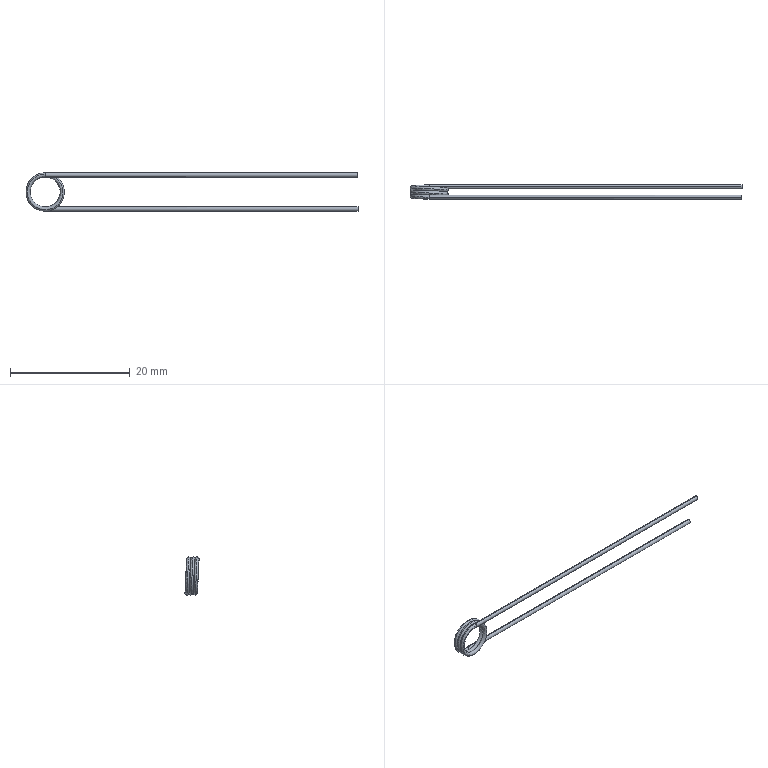Part | SolidWorks | features MoveFace 2, CompositeCurve 1, Helix 1, Sweep 1 | 1 solid | 9 faces | box 55.45 x 2.45 x 6.4 mm | volume 56.865 mm3 | cylinder 4 | spline 3 | plane 2 | commonest cylinder face diameters 0.7 x4
STEP:
#1=CARTESIAN_POINT('',(52.25,1.75,-3.2));
#2=VERTEX_POINT('',#1);
#3=CARTESIAN_POINT('',(52.25,1.75,-2.5));
#4=VERTEX_POINT('',#3);
#5=CARTESIAN_POINT('',(52.25,1.75,-2.85));
#6=DIRECTION('',(1.,0.,0.));
#7=DIRECTION('',(0.,0.00009155,-1.));
#8=AXIS2_PLACEMENT_3D('',#5,#6,#7);
#9=CIRCLE('',#8,0.35);
#10=EDGE_CURVE('',#2,#4,#9,.T.);
#11=ORIENTED_EDGE('',*,*,#10,.F.);
#12=CARTESIAN_POINT('',(-0.000000536,1.75,-3.2));
#13=VERTEX_POINT('',#12);
#14=CARTESIAN_POINT('',(12.85,1.75,-3.2));
#15=DIRECTION('',(-1.,0.,0.));
#16=VECTOR('',#15,1000.);
#17=LINE('',#14,#16);
#18=EDGE_CURVE('',#2,#13,#17,.T.);
#19=ORIENTED_EDGE('',*,*,#18,.T.);
#20=CARTESIAN_POINT('',(-0.006305,2.074,-2.979));
#21=VERTEX_POINT('',#20);
#22=CARTESIAN_POINT('',(0.,1.75,-2.85));
#23=DIRECTION('',(1.,0.,0.));
#24=DIRECTION('',(0.,0.00009155,-1.));
#25=AXIS2_PLACEMENT_3D('',#22,#23,#24);
#26=CIRCLE('',#25,0.35);
#27=EDGE_CURVE('',#13,#21,#26,.T.);
#28=ORIENTED_EDGE('',*,*,#27,.T.);
#29=CARTESIAN_POINT('',(0.,1.75,-2.5));
#30=VERTEX_POINT('',#29);
#31=CARTESIAN_POINT('',(0.,1.75,-2.85));
#32=DIRECTION('',(1.,0.,0.));
#33=DIRECTION('',(0.,0.00009155,-1.));
#34=AXIS2_PLACEMENT_3D('',#31,#32,#33);
#35=CIRCLE('',#34,0.35);
#36=EDGE_CURVE('',#21,#30,#35,.T.);
#37=ORIENTED_EDGE('',*,*,#36,.T.);
#38=CARTESIAN_POINT('',(12.85,1.75,-2.5));
#39=DIRECTION('',(-1.,0.,0.));
#40=VECTOR('',#39,1000.);
#41=LINE('',#38,#40);
#42=EDGE_CURVE('',#4,#30,#41,.T.);
#43=ORIENTED_EDGE('',*,*,#42,.F.);
#44=EDGE_LOOP('',(#11,#19,#28,#37,#43));
#45=FACE_OUTER_BOUND('',#44,.T.);
#46=CARTESIAN_POINT('',(12.85,1.75,-2.85));
#47=DIRECTION('',(-1.,0.,0.));
#48=DIRECTION('',(0.,0.,1.));
#49=AXIS2_PLACEMENT_3D('',#46,#47,#48);
#50=CYLINDRICAL_SURFACE('',#49,0.35);
#51=ADVANCED_FACE('',(#45),#50,.T.);
#52=CARTESIAN_POINT('',(0.006305,0.3239,2.979));
#53=VERTEX_POINT('',#52);
#54=CARTESIAN_POINT('',(0.,0.,3.2));
#55=VERTEX_POINT('',#54);
#56=CARTESIAN_POINT('',(0.006305,0.3239,2.979));
#57=CARTESIAN_POINT('',(0.01048,0.2681,3.104));
#58=CARTESIAN_POINT('',(0.005425,0.1388,3.2));
#59=CARTESIAN_POINT('',(0.,0.,3.2));
#60=B_SPLINE_CURVE_WITH_KNOTS('',3,(#56,#57,#58,#59),.UNSPECIFIED.,.F.,.F.,(4,4),(0.00002721,0.1895),.UNSPECIFIED.);
#61=EDGE_CURVE('',#53,#55,#60,.T.);
#62=ORIENTED_EDGE('',*,*,#61,.T.);
#63=CARTESIAN_POINT('',(52.25,0.,3.2));
#64=VERTEX_POINT('',#63);
#65=CARTESIAN_POINT('',(0.,0.,3.2));
#66=DIRECTION('',(1.,0.,0.));
#67=VECTOR('',#66,1000.);
#68=LINE('',#65,#67);
#69=EDGE_CURVE('',#55,#64,#68,.T.);
#70=ORIENTED_EDGE('',*,*,#69,.T.);
#71=CARTESIAN_POINT('',(52.25,0.,2.5));
#72=VERTEX_POINT('',#71);
#73=CARTESIAN_POINT('',(52.25,0.,2.85));
#74=DIRECTION('',(-1.,0.,0.));
#75=DIRECTION('',(0.,0.,1.));
#76=AXIS2_PLACEMENT_3D('',#73,#74,#75);
#77=CIRCLE('',#76,0.35);
#78=EDGE_CURVE('',#64,#72,#77,.T.);
#79=ORIENTED_EDGE('',*,*,#78,.T.);
#80=CARTESIAN_POINT('',(0.,0.,2.5));
#81=VERTEX_POINT('',#80);
#82=CARTESIAN_POINT('',(0.,0.,2.5));
#83=DIRECTION('',(1.,0.,0.));
#84=VECTOR('',#83,1000.);
#85=LINE('',#82,#84);
#86=EDGE_CURVE('',#81,#72,#85,.T.);
#87=ORIENTED_EDGE('',*,*,#86,.F.);
#88=CARTESIAN_POINT('',(0.,0.,2.85));
#89=DIRECTION('',(-1.,0.,0.));
#90=DIRECTION('',(0.,0.,1.));
#91=AXIS2_PLACEMENT_3D('',#88,#89,#90);
#92=CIRCLE('',#91,0.35);
#93=EDGE_CURVE('',#53,#81,#92,.T.);
#94=ORIENTED_EDGE('',*,*,#93,.F.);
#95=EDGE_LOOP('',(#62,#70,#79,#87,#94));
#96=FACE_OUTER_BOUND('',#95,.T.);
#97=CARTESIAN_POINT('',(0.,0.,2.85));
#98=DIRECTION('',(1.,0.,0.));
#99=DIRECTION('',(0.,0.,-1.));
#100=AXIS2_PLACEMENT_3D('',#97,#98,#99);
#101=CYLINDRICAL_SURFACE('',#100,0.35);
#102=ADVANCED_FACE('',(#96),#101,.T.);
#103=ORIENTED_EDGE('',*,*,#18,.F.);
#104=CARTESIAN_POINT('',(52.25,1.75,-2.85));
#105=DIRECTION('',(1.,0.,0.));
#106=DIRECTION('',(0.,0.00009155,-1.));
#107=AXIS2_PLACEMENT_3D('',#104,#105,#106);
#108=CIRCLE('',#107,0.35);
#109=EDGE_CURVE('',#4,#2,#108,.T.);
#110=ORIENTED_EDGE('',*,*,#109,.F.);
#111=ORIENTED_EDGE('',*,*,#42,.T.);
#112=CARTESIAN_POINT('',(0.006304,1.426,-2.979));
#113=VERTEX_POINT('',#112);
#114=CARTESIAN_POINT('',(0.,1.75,-2.85));
#115=DIRECTION('',(1.,0.,0.));
#116=DIRECTION('',(0.,0.00009155,-1.));
#117=AXIS2_PLACEMENT_3D('',#114,#115,#116);
#118=CIRCLE('',#117,0.35);
#119=EDGE_CURVE('',#30,#113,#118,.T.);
#120=ORIENTED_EDGE('',*,*,#119,.T.);
#121=CARTESIAN_POINT('',(0.,1.75,-2.85));
#122=DIRECTION('',(1.,0.,0.));
#123=DIRECTION('',(0.,0.00009155,-1.));
#124=AXIS2_PLACEMENT_3D('',#121,#122,#123);
#125=CIRCLE('',#124,0.35);
#126=EDGE_CURVE('',#113,#13,#125,.T.);
#127=ORIENTED_EDGE('',*,*,#126,.T.);
#128=EDGE_LOOP('',(#103,#110,#111,#120,#127));
#129=FACE_OUTER_BOUND('',#128,.T.);
#130=CARTESIAN_POINT('',(12.85,1.75,-2.85));
#131=DIRECTION('',(-1.,0.,0.));
#132=DIRECTION('',(0.,0.,1.));
#133=AXIS2_PLACEMENT_3D('',#130,#131,#132);
#134=CYLINDRICAL_SURFACE('',#133,0.35);
#135=ADVANCED_FACE('',(#129),#134,.T.);
#136=ORIENTED_EDGE('',*,*,#36,.F.);
#137=CARTESIAN_POINT('',(0.006305,0.3239,2.979));
#138=CARTESIAN_POINT('',(-0.7712,0.3519,2.981));
#139=CARTESIAN_POINT('',(-1.545,0.381,2.663));
#140=CARTESIAN_POINT('',(-2.649,0.4392,1.566));
#141=CARTESIAN_POINT('',(-2.975,0.4683,0.7939));
#142=CARTESIAN_POINT('',(-2.98,0.5195,-0.5733));
#143=CARTESIAN_POINT('',(-2.806,0.5413,-1.156));
#144=CARTESIAN_POINT('',(-2.162,0.585,-2.13));
#145=CARTESIAN_POINT('',(-1.69,0.6069,-2.521));
#146=CARTESIAN_POINT('',(-0.4324,0.658,-3.048));
#147=CARTESIAN_POINT('',(0.405,0.6871,-3.052));
#148=CARTESIAN_POINT('',(1.67,0.7383,-2.534));
#149=CARTESIAN_POINT('',(2.142,0.7601,-2.15));
#150=CARTESIAN_POINT('',(2.795,0.8037,-1.182));
#151=CARTESIAN_POINT('',(2.976,0.8257,-0.5972));
#152=CARTESIAN_POINT('',(2.981,0.8768,0.7668));
#153=CARTESIAN_POINT('',(2.665,0.9058,1.542));
#154=CARTESIAN_POINT('',(1.702,0.957,2.513));
#155=CARTESIAN_POINT('',(1.167,0.9788,2.801));
#156=CARTESIAN_POINT('',(0.02248,1.022,3.035));
#157=CARTESIAN_POINT('',(-0.587,1.044,2.978));
#158=CARTESIAN_POINT('',(-1.849,1.096,2.461));
#159=CARTESIAN_POINT('',(-2.445,1.125,1.872));
#160=CARTESIAN_POINT('',(-2.973,1.176,0.6109));
#161=CARTESIAN_POINT('',(-3.035,1.198,0.005944));
#162=CARTESIAN_POINT('',(-2.812,1.241,-1.14));
#163=CARTESIAN_POINT('',(-2.526,1.263,-1.682));
#164=CARTESIAN_POINT('',(-1.566,1.314,-2.65));
#165=CARTESIAN_POINT('',(-0.7938,1.343,-2.975));
#166=CARTESIAN_POINT('',(0.5733,1.395,-2.98));
#167=CARTESIAN_POINT('',(1.156,1.416,-2.806));
#168=CARTESIAN_POINT('',(2.13,1.46,-2.162));
#169=CARTESIAN_POINT('',(2.521,1.482,-1.69));
#170=CARTESIAN_POINT('',(3.048,1.533,-0.4324));
#171=CARTESIAN_POINT('',(3.052,1.562,0.405));
#172=CARTESIAN_POINT('',(2.534,1.613,1.67));
#173=CARTESIAN_POINT('',(2.15,1.635,2.142));
#174=CARTESIAN_POINT('',(1.182,1.679,2.795));
#175=CARTESIAN_POINT('',(0.5972,1.701,2.976));
#176=CARTESIAN_POINT('',(-0.7668,1.752,2.981));
#177=CARTESIAN_POINT('',(-1.542,1.781,2.665));
#178=CARTESIAN_POINT('',(-2.513,1.832,1.702));
#179=CARTESIAN_POINT('',(-2.801,1.854,1.167));
#180=CARTESIAN_POINT('',(-3.034,1.897,0.0225));
#181=CARTESIAN_POINT('',(-2.978,1.919,-0.587));
#182=CARTESIAN_POINT('',(-2.46,1.971,-1.85));
#183=CARTESIAN_POINT('',(-1.872,2.,-2.445));
#184=CARTESIAN_POINT('',(-0.7917,2.043,-2.897));
#185=CARTESIAN_POINT('',(-0.4042,2.058,-2.976));
#186=CARTESIAN_POINT('',(-0.006305,2.074,-2.979));
#187=B_SPLINE_CURVE_WITH_KNOTS('',3,(#137,#138,#139,#140,#141,#142,#143,#144,#145,#146,#147,#148,#149,#150,#151,#152,#153,#154,#155,#156,#157,#158,#159,#160,#161,#162,#163,#164,#165,#166,#167,#168,#169,#170,#171,#172,#173,#174,#175,#176,#177,#178,#179,#180,#181,#182,#183,#184,#185,#186),.UNSPECIFIED.,.F.,.F.,(4,2,2,2,2,2,2,2,2,2,2,2,2,2,2,2,2,2,2,2,2,2,2,2,4),(0.,0.04998,0.09999,0.1375,0.175,0.225,0.2625,0.3,0.35,0.3875,0.425,0.475,0.5125,0.55,0.6,0.6375,0.675,0.725,0.7625,0.8,0.85,0.8875,0.925,0.975,1.),.UNSPECIFIED.);
#188=EDGE_CURVE('',#53,#21,#187,.T.);
#189=ORIENTED_EDGE('',*,*,#188,.F.);
#190=ORIENTED_EDGE('',*,*,#93,.T.);
#191=CARTESIAN_POINT('',(-0.006304,-0.3239,2.979));
#192=VERTEX_POINT('',#191);
#193=CARTESIAN_POINT('',(0.,0.,2.85));
#194=DIRECTION('',(-1.,0.,0.));
#195=DIRECTION('',(0.,0.,1.));
#196=AXIS2_PLACEMENT_3D('',#193,#194,#195);
#197=CIRCLE('',#196,0.35);
#198=EDGE_CURVE('',#81,#192,#197,.T.);
#199=ORIENTED_EDGE('',*,*,#198,.T.);
#200=CARTESIAN_POINT('',(0.006304,1.426,-2.979));
#201=CARTESIAN_POINT('',(-0.379,1.413,-2.98));
#202=CARTESIAN_POINT('',(-0.7673,1.398,-2.904));
#203=CARTESIAN_POINT('',(-1.851,1.354,-2.461));
#204=CARTESIAN_POINT('',(-2.445,1.325,-1.871));
#205=CARTESIAN_POINT('',(-2.973,1.274,-0.6122));
#206=CARTESIAN_POINT('',(-3.035,1.252,-0.003211));
#207=CARTESIAN_POINT('',(-2.811,1.209,1.143));
#208=CARTESIAN_POINT('',(-2.527,1.187,1.681));
#209=CARTESIAN_POINT('',(-1.565,1.136,2.652));
#210=CARTESIAN_POINT('',(-0.792,1.107,2.975));
#211=CARTESIAN_POINT('',(0.572,1.056,2.981));
#212=CARTESIAN_POINT('',(1.158,1.034,2.805));
#213=CARTESIAN_POINT('',(2.132,0.99,2.16));
#214=CARTESIAN_POINT('',(2.52,0.9682,1.692));
#215=CARTESIAN_POINT('',(3.049,0.917,0.4308));
#216=CARTESIAN_POINT('',(3.052,0.8879,-0.4067));
#217=CARTESIAN_POINT('',(2.535,0.8368,-1.669));
#218=CARTESIAN_POINT('',(2.148,0.8149,-2.144));
#219=CARTESIAN_POINT('',(1.18,0.7712,-2.796));
#220=CARTESIAN_POINT('',(0.5985,0.7494,-2.976));
#221=CARTESIAN_POINT('',(-0.7686,0.6982,-2.981));
#222=CARTESIAN_POINT('',(-1.544,0.6692,-2.664));
#223=CARTESIAN_POINT('',(-2.512,0.6181,-1.703));
#224=CARTESIAN_POINT('',(-2.802,0.5961,-1.164));
#225=CARTESIAN_POINT('',(-3.035,0.5525,-0.01977));
#226=CARTESIAN_POINT('',(-2.978,0.5307,0.5858));
#227=CARTESIAN_POINT('',(-2.46,0.4795,1.851));
#228=CARTESIAN_POINT('',(-1.87,0.4504,2.445));
#229=CARTESIAN_POINT('',(-0.6122,0.3993,2.973));
#230=CARTESIAN_POINT('',(-0.003226,0.3774,3.035));
#231=CARTESIAN_POINT('',(1.143,0.3337,2.811));
#232=CARTESIAN_POINT('',(1.681,0.3119,2.527));
#233=CARTESIAN_POINT('',(2.652,0.2607,1.565));
#234=CARTESIAN_POINT('',(2.975,0.2317,0.792));
#235=CARTESIAN_POINT('',(2.981,0.1806,-0.572));
#236=CARTESIAN_POINT('',(2.805,0.1586,-1.158));
#237=CARTESIAN_POINT('',(2.16,0.115,-2.132));
#238=CARTESIAN_POINT('',(1.692,0.09317,-2.52));
#239=CARTESIAN_POINT('',(0.4308,0.04196,-3.049));
#240=CARTESIAN_POINT('',(-0.4067,0.01292,-3.052));
#241=CARTESIAN_POINT('',(-1.669,-0.03818,-2.535));
#242=CARTESIAN_POINT('',(-2.144,-0.06013,-2.148));
#243=CARTESIAN_POINT('',(-2.796,-0.1038,-1.18));
#244=CARTESIAN_POINT('',(-2.976,-0.1256,-0.5985));
#245=CARTESIAN_POINT('',(-2.981,-0.1768,0.7687));
#246=CARTESIAN_POINT('',(-2.663,-0.2059,1.544));
#247=CARTESIAN_POINT('',(-1.567,-0.2642,2.65));
#248=CARTESIAN_POINT('',(-0.7966,-0.2932,2.975));
#249=CARTESIAN_POINT('',(-0.006304,-0.3239,2.979));
#250=B_SPLINE_CURVE_WITH_KNOTS('',3,(#200,#201,#202,#203,#204,#205,#206,#207,#208,#209,#210,#211,#212,#213,#214,#215,#216,#217,#218,#219,#220,#221,#222,#223,#224,#225,#226,#227,#228,#229,#230,#231,#232,#233,#234,#235,#236,#237,#238,#239,#240,#241,#242,#243,#244,#245,#246,#247,#248,#249),.UNSPECIFIED.,.F.,.F.,(4,2,2,2,2,2,2,2,2,2,2,2,2,2,2,2,2,2,2,2,2,2,2,2,4),(0.,0.02496,0.07501,0.1125,0.15,0.2,0.2375,0.275,0.325,0.3625,0.4,0.45,0.4875,0.525,0.575,0.6125,0.65,0.7,0.7375,0.775,0.825,0.8625,0.9,0.95,1.),.UNSPECIFIED.);
#251=EDGE_CURVE('',#113,#192,#250,.T.);
#252=ORIENTED_EDGE('',*,*,#251,.F.);
#253=ORIENTED_EDGE('',*,*,#119,.F.);
#254=EDGE_LOOP('',(#136,#189,#190,#199,#252,#253));
#255=FACE_OUTER_BOUND('',#254,.T.);
#256=CARTESIAN_POINT('',(-0.01261,2.073,-2.978));
#257=CARTESIAN_POINT('',(-0.9931,2.036,-2.974));
#258=CARTESIAN_POINT('',(-1.942,2.,-2.452));
#259=CARTESIAN_POINT('',(-3.022,1.927,-0.8338));
#260=CARTESIAN_POINT('',(-3.123,1.89,0.2539));
#261=CARTESIAN_POINT('',(-2.369,1.817,2.048));
#262=CARTESIAN_POINT('',(-1.523,1.781,2.732));
#263=CARTESIAN_POINT('',(0.3864,1.708,3.111));
#264=CARTESIAN_POINT('',(1.43,1.671,2.788));
#265=CARTESIAN_POINT('',(2.798,1.599,1.405));
#266=CARTESIAN_POINT('',(3.107,1.562,0.3615));
#267=CARTESIAN_POINT('',(2.726,1.489,-1.547));
#268=CARTESIAN_POINT('',(2.029,1.453,-2.388));
#269=CARTESIAN_POINT('',(0.2273,1.38,-3.123));
#270=CARTESIAN_POINT('',(-0.8551,1.343,-3.009));
#271=CARTESIAN_POINT('',(-2.473,1.271,-1.927));
#272=CARTESIAN_POINT('',(-2.982,1.234,-0.9604));
#273=CARTESIAN_POINT('',(-2.972,1.161,0.9852));
#274=CARTESIAN_POINT('',(-2.453,1.125,1.942));
#275=CARTESIAN_POINT('',(-0.8335,1.052,3.022));
#276=CARTESIAN_POINT('',(0.2539,1.015,3.123));
#277=CARTESIAN_POINT('',(2.048,0.9425,2.369));
#278=CARTESIAN_POINT('',(2.732,0.9059,1.523));
#279=CARTESIAN_POINT('',(3.111,0.8331,-0.3864));
#280=CARTESIAN_POINT('',(2.788,0.7965,-1.43));
#281=CARTESIAN_POINT('',(1.405,0.7237,-2.798));
#282=CARTESIAN_POINT('',(0.3615,0.6872,-3.107));
#283=CARTESIAN_POINT('',(-1.547,0.6143,-2.726));
#284=CARTESIAN_POINT('',(-2.388,0.5777,-2.029));
#285=CARTESIAN_POINT('',(-3.123,0.505,-0.2273));
#286=CARTESIAN_POINT('',(-3.009,0.4684,0.8554));
#287=CARTESIAN_POINT('',(-1.927,0.3956,2.473));
#288=CARTESIAN_POINT('',(-0.9676,0.3593,2.982));
#289=CARTESIAN_POINT('',(0.01261,0.3226,2.978));
#290=CARTESIAN_POINT('',(-0.0161,2.162,-2.771));
#291=CARTESIAN_POINT('',(-0.9269,2.125,-2.766));
#292=CARTESIAN_POINT('',(-1.811,2.089,-2.279));
#293=CARTESIAN_POINT('',(-2.813,2.016,-0.7712));
#294=CARTESIAN_POINT('',(-2.906,1.979,0.2409));
#295=CARTESIAN_POINT('',(-2.201,1.907,1.909));
#296=CARTESIAN_POINT('',(-1.413,1.87,2.545));
#297=CARTESIAN_POINT('',(0.3644,1.797,2.894));
#298=CARTESIAN_POINT('',(1.334,1.761,2.592));
#299=CARTESIAN_POINT('',(2.606,1.688,1.303));
#300=CARTESIAN_POINT('',(2.892,1.651,0.3318));
#301=CARTESIAN_POINT('',(2.535,1.579,-1.444));
#302=CARTESIAN_POINT('',(1.884,1.542,-2.225));
#303=CARTESIAN_POINT('',(0.2064,1.469,-2.907));
#304=CARTESIAN_POINT('',(-0.8001,1.433,-2.799));
#305=CARTESIAN_POINT('',(-2.304,1.36,-1.789));
#306=CARTESIAN_POINT('',(-2.777,1.323,-0.8894));
#307=CARTESIAN_POINT('',(-2.764,1.25,0.9216));
#308=CARTESIAN_POINT('',(-2.279,1.214,1.81));
#309=CARTESIAN_POINT('',(-0.771,1.141,2.814));
#310=CARTESIAN_POINT('',(0.2409,1.104,2.906));
#311=CARTESIAN_POINT('',(1.909,1.032,2.201));
#312=CARTESIAN_POINT('',(2.545,0.9951,1.413));
#313=CARTESIAN_POINT('',(2.894,0.9223,-0.3644));
#314=CARTESIAN_POINT('',(2.592,0.8857,-1.334));
#315=CARTESIAN_POINT('',(1.303,0.8129,-2.606));
#316=CARTESIAN_POINT('',(0.3318,0.7764,-2.892));
#317=CARTESIAN_POINT('',(-1.444,0.7035,-2.535));
#318=CARTESIAN_POINT('',(-2.225,0.667,-1.884));
#319=CARTESIAN_POINT('',(-2.907,0.5942,-0.2064));
#320=CARTESIAN_POINT('',(-2.798,0.5576,0.8003));
#321=CARTESIAN_POINT('',(-1.789,0.4848,2.304));
#322=CARTESIAN_POINT('',(-0.8958,0.4485,2.776));
#323=CARTESIAN_POINT('',(0.0161,0.4118,2.771));
#324=CARTESIAN_POINT('',(-0.008888,1.977,-2.5));
#325=CARTESIAN_POINT('',(-0.8283,1.941,-2.497));
#326=CARTESIAN_POINT('',(-1.629,1.904,-2.059));
#327=CARTESIAN_POINT('',(-2.536,1.832,-0.7012));
#328=CARTESIAN_POINT('',(-2.622,1.795,0.2114));
#329=CARTESIAN_POINT('',(-1.989,1.722,1.718));
#330=CARTESIAN_POINT('',(-1.28,1.686,2.292));
#331=CARTESIAN_POINT('',(0.3232,1.613,2.612));
#332=CARTESIAN_POINT('',(1.199,1.576,2.341));
#333=CARTESIAN_POINT('',(2.349,1.503,1.18));
#334=CARTESIAN_POINT('',(2.608,1.467,0.3051));
#335=CARTESIAN_POINT('',(2.29,1.394,-1.298));
#336=CARTESIAN_POINT('',(1.704,1.358,-2.003));
#337=CARTESIAN_POINT('',(0.1914,1.285,-2.622));
#338=CARTESIAN_POINT('',(-0.716,1.248,-2.526));
#339=CARTESIAN_POINT('',(-2.075,1.175,-1.618));
#340=CARTESIAN_POINT('',(-2.503,1.139,-0.808));
#341=CARTESIAN_POINT('',(-2.495,1.066,0.8264));
#342=CARTESIAN_POINT('',(-2.06,1.029,1.628));
#343=CARTESIAN_POINT('',(-0.701,0.9565,2.537));
#344=CARTESIAN_POINT('',(0.2114,0.92,2.622));
#345=CARTESIAN_POINT('',(1.718,0.8471,1.989));
#346=CARTESIAN_POINT('',(2.292,0.8107,1.28));
#347=CARTESIAN_POINT('',(2.612,0.7378,-0.3232));
#348=CARTESIAN_POINT('',(2.341,0.7013,-1.199));
#349=CARTESIAN_POINT('',(1.18,0.6284,-2.349));
#350=CARTESIAN_POINT('',(0.3051,0.5919,-2.608));
#351=CARTESIAN_POINT('',(-1.298,0.519,-2.29));
#352=CARTESIAN_POINT('',(-2.003,0.4825,-1.704));
#353=CARTESIAN_POINT('',(-2.622,0.4096,-0.1914));
#354=CARTESIAN_POINT('',(-2.525,0.3732,0.7162));
#355=CARTESIAN_POINT('',(-1.619,0.3003,2.075));
#356=CARTESIAN_POINT('',(-0.8134,0.2639,2.503));
#357=CARTESIAN_POINT('',(0.008889,0.2274,2.5));
#358=CARTESIAN_POINT('',(0.008895,1.522,-2.5));
#359=CARTESIAN_POINT('',(-0.8105,1.486,-2.503));
#360=CARTESIAN_POINT('',(-1.614,1.45,-2.071));
#361=CARTESIAN_POINT('',(-2.532,1.377,-0.7193));
#362=CARTESIAN_POINT('',(-2.623,1.34,0.1927));
#363=CARTESIAN_POINT('',(-2.001,1.267,1.704));
#364=CARTESIAN_POINT('',(-1.296,1.231,2.283));
#365=CARTESIAN_POINT('',(0.3046,1.158,2.614));
#366=CARTESIAN_POINT('',(1.182,1.121,2.35));
#367=CARTESIAN_POINT('',(2.341,1.048,1.197));
#368=CARTESIAN_POINT('',(2.606,1.012,0.3236));
#369=CARTESIAN_POINT('',(2.299,0.9391,-1.282));
#370=CARTESIAN_POINT('',(1.719,0.9026,-1.991));
#371=CARTESIAN_POINT('',(0.2101,0.8297,-2.62));
#372=CARTESIAN_POINT('',(-0.6981,0.7933,-2.531));
#373=CARTESIAN_POINT('',(-2.064,0.7204,-1.633));
#374=CARTESIAN_POINT('',(-2.497,0.6839,-0.8259));
#375=CARTESIAN_POINT('',(-2.501,0.611,0.8087));
#376=CARTESIAN_POINT('',(-2.071,0.5745,1.614));
#377=CARTESIAN_POINT('',(-0.7191,0.5016,2.532));
#378=CARTESIAN_POINT('',(0.1927,0.4651,2.623));
#379=CARTESIAN_POINT('',(1.704,0.3922,2.001));
#380=CARTESIAN_POINT('',(2.283,0.3558,1.296));
#381=CARTESIAN_POINT('',(2.614,0.2829,-0.3046));
#382=CARTESIAN_POINT('',(2.35,0.2464,-1.182));
#383=CARTESIAN_POINT('',(1.197,0.1735,-2.341));
#384=CARTESIAN_POINT('',(0.3236,0.137,-2.606));
#385=CARTESIAN_POINT('',(-1.282,0.0641,-2.299));
#386=CARTESIAN_POINT('',(-1.991,0.02763,-1.719));
#387=CARTESIAN_POINT('',(-2.62,-0.04528,-0.2101));
#388=CARTESIAN_POINT('',(-2.531,-0.08173,0.6983));
#389=CARTESIAN_POINT('',(-1.633,-0.1546,2.064));
#390=CARTESIAN_POINT('',(-0.8313,-0.191,2.497));
#391=CARTESIAN_POINT('',(-0.008894,-0.2275,2.5));
#392=CARTESIAN_POINT('',(0.0161,1.338,-2.771));
#393=CARTESIAN_POINT('',(-0.8947,1.302,-2.777));
#394=CARTESIAN_POINT('',(-1.785,1.265,-2.3));
#395=CARTESIAN_POINT('',(-2.804,1.192,-0.804));
#396=CARTESIAN_POINT('',(-2.908,1.156,0.2071));
#397=CARTESIAN_POINT('',(-2.223,1.083,1.884));
#398=CARTESIAN_POINT('',(-1.443,1.046,2.528));
#399=CARTESIAN_POINT('',(0.3307,0.9736,2.899));
#400=CARTESIAN_POINT('',(1.304,0.937,2.608));
#401=CARTESIAN_POINT('',(2.591,0.8642,1.333));
#402=CARTESIAN_POINT('',(2.888,0.8277,0.3653));
#403=CARTESIAN_POINT('',(2.552,0.7548,-1.415));
#404=CARTESIAN_POINT('',(1.91,0.7183,-2.203));
#405=CARTESIAN_POINT('',(0.2402,0.6455,-2.904));
#406=CARTESIAN_POINT('',(-0.7677,0.6089,-2.808));
#407=CARTESIAN_POINT('',(-2.284,0.5361,-1.816));
#408=CARTESIAN_POINT('',(-2.766,0.4995,-0.9217));
#409=CARTESIAN_POINT('',(-2.775,0.4267,0.8895));
#410=CARTESIAN_POINT('',(-2.3,0.3902,1.784));
#411=CARTESIAN_POINT('',(-0.8038,0.3173,2.805));
#412=CARTESIAN_POINT('',(0.2071,0.2808,2.908));
#413=CARTESIAN_POINT('',(1.884,0.208,2.223));
#414=CARTESIAN_POINT('',(2.528,0.1714,1.443));
#415=CARTESIAN_POINT('',(2.899,0.09857,-0.3307));
#416=CARTESIAN_POINT('',(2.608,0.06204,-1.304));
#417=CARTESIAN_POINT('',(1.333,-0.01079,-2.591));
#418=CARTESIAN_POINT('',(0.3653,-0.0473,-2.888));
#419=CARTESIAN_POINT('',(-1.415,-0.1202,-2.552));
#420=CARTESIAN_POINT('',(-2.203,-0.1567,-1.91));
#421=CARTESIAN_POINT('',(-2.904,-0.2295,-0.2402));
#422=CARTESIAN_POINT('',(-2.807,-0.2661,0.7679));
#423=CARTESIAN_POINT('',(-1.816,-0.3389,2.283));
#424=CARTESIAN_POINT('',(-0.9282,-0.3752,2.766));
#425=CARTESIAN_POINT('',(-0.0161,-0.4119,2.771));
#426=CARTESIAN_POINT('',(0.01261,1.427,-2.978));
#427=CARTESIAN_POINT('',(-0.9679,1.391,-2.982));
#428=CARTESIAN_POINT('',(-1.922,1.354,-2.469));
#429=CARTESIAN_POINT('',(-3.015,1.282,-0.8595));
#430=CARTESIAN_POINT('',(-3.125,1.245,0.2275));
#431=CARTESIAN_POINT('',(-2.386,1.172,2.028));
#432=CARTESIAN_POINT('',(-1.546,1.136,2.72));
#433=CARTESIAN_POINT('',(0.36,1.063,3.114));
#434=CARTESIAN_POINT('',(1.406,1.026,2.8));
#435=CARTESIAN_POINT('',(2.787,0.9536,1.429));
#436=CARTESIAN_POINT('',(3.104,0.917,0.3878));
#437=CARTESIAN_POINT('',(2.739,0.8442,-1.524));
#438=CARTESIAN_POINT('',(2.049,0.8076,-2.37));
#439=CARTESIAN_POINT('',(0.2537,0.7349,-3.121));
#440=CARTESIAN_POINT('',(-0.8297,0.6983,-3.016));
#441=CARTESIAN_POINT('',(-2.457,0.6254,-1.948));
#442=CARTESIAN_POINT('',(-2.974,0.5889,-0.9857));
#443=CARTESIAN_POINT('',(-2.981,0.5161,0.96));
#444=CARTESIAN_POINT('',(-2.469,0.4795,1.921));
#445=CARTESIAN_POINT('',(-0.8592,0.4067,3.015));
#446=CARTESIAN_POINT('',(0.2275,0.3701,3.125));
#447=CARTESIAN_POINT('',(2.028,0.2974,2.386));
#448=CARTESIAN_POINT('',(2.72,0.2608,1.546));
#449=CARTESIAN_POINT('',(3.114,0.1879,-0.36));
#450=CARTESIAN_POINT('',(2.8,0.1514,-1.406));
#451=CARTESIAN_POINT('',(1.429,0.07861,-2.787));
#452=CARTESIAN_POINT('',(0.3878,0.04204,-3.104));
#453=CARTESIAN_POINT('',(-1.524,-0.03081,-2.739));
#454=CARTESIAN_POINT('',(-2.371,-0.06738,-2.049));
#455=CARTESIAN_POINT('',(-3.121,-0.1401,-0.2537));
#456=CARTESIAN_POINT('',(-3.016,-0.1767,0.83));
#457=CARTESIAN_POINT('',(-1.948,-0.2496,2.456));
#458=CARTESIAN_POINT('',(-0.993,-0.2858,2.974));
#459=CARTESIAN_POINT('',(-0.01261,-0.3225,2.978));
#460=B_SPLINE_SURFACE_WITH_KNOTS('',3,3,((#256,#257,#258,#259,#260,#261,#262,#263,#264,#265,#266,#267,#268,#269,#270,#271,#272,#273,#274,#275,#276,#277,#278,#279,#280,#281,#282,#283,#284,#285,#286,#287,#288,#289),(#290,#291,#292,#293,#294,#295,#296,#297,#298,#299,#300,#301,#302,#303,#304,#305,#306,#307,#308,#309,#310,#311,#312,#313,#314,#315,#316,#317,#318,#319,#320,#321,#322,#323),(#324,#325,#326,#327,#328,#329,#330,#331,#332,#333,#334,#335,#336,#337,#338,#339,#340,#341,#342,#343,#344,#345,#346,#347,#348,#349,#350,#351,#352,#353,#354,#355,#356,#357),(#358,#359,#360,#361,#362,#363,#364,#365,#366,#367,#368,#369,#370,#371,#372,#373,#374,#375,#376,#377,#378,#379,#380,#381,#382,#383,#384,#385,#386,#387,#388,#389,#390,#391),(#392,#393,#394,#395,#396,#397,#398,#399,#400,#401,#402,#403,#404,#405,#406,#407,#408,#409,#410,#411,#412,#413,#414,#415,#416,#417,#418,#419,#420,#421,#422,#423,#424,#425),(#426,#427,#428,#429,#430,#431,#432,#433,#434,#435,#436,#437,#438,#439,#440,#441,#442,#443,#444,#445,#446,#447,#448,#449,#450,#451,#452,#453,#454,#455,#456,#457,#458,#459)),.UNSPECIFIED.,.F.,.F.,.F.,(4,2,4),(4,2,2,2,2,2,2,2,2,2,2,2,2,2,2,2,4),(0.1895,0.5,0.8106),(0.,0.0625,0.125,0.1875,0.25,0.3125,0.375,0.4375,0.5,0.5625,0.625,0.6875,0.75,0.8125,0.875,0.9375,1.),.UNSPECIFIED.);
#461=ADVANCED_FACE('',(#255),#460,.F.);
#462=ORIENTED_EDGE('',*,*,#126,.F.);
#463=ORIENTED_EDGE('',*,*,#251,.T.);
#464=CARTESIAN_POINT('',(0.,0.,3.2));
#465=CARTESIAN_POINT('',(-0.005423,-0.1387,3.2));
#466=CARTESIAN_POINT('',(-0.01048,-0.268,3.104));
#467=CARTESIAN_POINT('',(-0.006304,-0.3239,2.979));
#468=B_SPLINE_CURVE_WITH_KNOTS('',3,(#464,#465,#466,#467),.UNSPECIFIED.,.F.,.F.,(4,4),(0.8106,1.),.UNSPECIFIED.);
#469=EDGE_CURVE('',#55,#192,#468,.T.);
#470=ORIENTED_EDGE('',*,*,#469,.F.);
#471=CARTESIAN_POINT('',(-0.000000536,1.75,-3.2));
#472=CARTESIAN_POINT('',(-0.4215,1.735,-3.2));
#473=CARTESIAN_POINT('',(-0.8371,1.721,-3.117));
#474=CARTESIAN_POINT('',(-2.001,1.677,-2.635));
#475=CARTESIAN_POINT('',(-2.635,1.648,-2.));
#476=CARTESIAN_POINT('',(-3.197,1.597,-0.6438));
#477=CARTESIAN_POINT('',(-3.261,1.575,0.01064));
#478=CARTESIAN_POINT('',(-3.015,1.531,1.241));
#479=CARTESIAN_POINT('',(-2.708,1.51,1.817));
#480=CARTESIAN_POINT('',(-1.669,1.458,2.857));
#481=CARTESIAN_POINT('',(-0.8382,1.429,3.2));
#482=CARTESIAN_POINT('',(0.6287,1.378,3.2));
#483=CARTESIAN_POINT('',(1.258,1.356,3.008));
#484=CARTESIAN_POINT('',(2.3,1.313,2.311));
#485=CARTESIAN_POINT('',(2.715,1.291,1.807));
#486=CARTESIAN_POINT('',(3.278,1.239,0.4484));
#487=CARTESIAN_POINT('',(3.277,1.211,-0.4502));
#488=CARTESIAN_POINT('',(2.716,1.159,-1.805));
#489=CARTESIAN_POINT('',(2.298,1.137,-2.313));
#490=CARTESIAN_POINT('',(1.255,1.094,-3.01));
#491=CARTESIAN_POINT('',(0.6301,1.072,-3.2));
#492=CARTESIAN_POINT('',(-0.8402,1.021,-3.2));
#493=CARTESIAN_POINT('',(-1.67,0.9918,-2.855));
#494=CARTESIAN_POINT('',(-2.707,0.9406,-1.818));
#495=CARTESIAN_POINT('',(-3.017,0.9186,-1.238));
#496=CARTESIAN_POINT('',(-3.261,0.875,-0.007701));
#497=CARTESIAN_POINT('',(-3.198,0.8533,0.6424));
#498=CARTESIAN_POINT('',(-2.635,0.8019,2.001));
#499=CARTESIAN_POINT('',(-1.999,0.773,2.636));
#500=CARTESIAN_POINT('',(-0.6438,0.7218,3.197));
#501=CARTESIAN_POINT('',(0.01062,0.6999,3.261));
#502=CARTESIAN_POINT('',(1.241,0.6563,3.015));
#503=CARTESIAN_POINT('',(1.817,0.6345,2.708));
#504=CARTESIAN_POINT('',(2.857,0.5832,1.669));
#505=CARTESIAN_POINT('',(3.2,0.5543,0.8382));
#506=CARTESIAN_POINT('',(3.2,0.5031,-0.6287));
#507=CARTESIAN_POINT('',(3.008,0.4811,-1.258));
#508=CARTESIAN_POINT('',(2.311,0.4375,-2.3));
#509=CARTESIAN_POINT('',(1.807,0.4158,-2.715));
#510=CARTESIAN_POINT('',(0.4484,0.3644,-3.278));
#511=CARTESIAN_POINT('',(-0.4502,0.3355,-3.277));
#512=CARTESIAN_POINT('',(-1.805,0.2843,-2.716));
#513=CARTESIAN_POINT('',(-2.313,0.2624,-2.298));
#514=CARTESIAN_POINT('',(-3.01,0.2188,-1.255));
#515=CARTESIAN_POINT('',(-3.2,0.197,-0.6301));
#516=CARTESIAN_POINT('',(-3.2,0.1457,0.8403));
#517=CARTESIAN_POINT('',(-2.854,0.1167,1.671));
#518=CARTESIAN_POINT('',(-1.671,0.05831,2.854));
#519=CARTESIAN_POINT('',(-0.8425,0.02943,3.2));
#520=CARTESIAN_POINT('',(0.,0.,3.2));
#521=B_SPLINE_CURVE_WITH_KNOTS('',3,(#471,#472,#473,#474,#475,#476,#477,#478,#479,#480,#481,#482,#483,#484,#485,#486,#487,#488,#489,#490,#491,#492,#493,#494,#495,#496,#497,#498,#499,#500,#501,#502,#503,#504,#505,#506,#507,#508,#509,#510,#511,#512,#513,#514,#515,#516,#517,#518,#519,#520),.UNSPECIFIED.,.F.,.F.,(4,2,2,2,2,2,2,2,2,2,2,2,2,2,2,2,2,2,2,2,2,2,2,2,4),(0.,0.02496,0.07501,0.1125,0.15,0.2,0.2375,0.275,0.325,0.3625,0.4,0.45,0.4875,0.525,0.575,0.6125,0.65,0.7,0.7375,0.775,0.825,0.8625,0.9,0.95,1.),.UNSPECIFIED.);
#522=EDGE_CURVE('',#13,#55,#521,.T.);
#523=ORIENTED_EDGE('',*,*,#522,.F.);
#524=EDGE_LOOP('',(#462,#463,#470,#523));
#525=FACE_OUTER_BOUND('',#524,.T.);
#526=CARTESIAN_POINT('',(0.01261,1.427,-2.978));
#527=CARTESIAN_POINT('',(-0.379,1.413,-2.98));
#528=CARTESIAN_POINT('',(-0.7673,1.398,-2.904));
#529=CARTESIAN_POINT('',(-1.851,1.354,-2.461));
#530=CARTESIAN_POINT('',(-2.445,1.325,-1.871));
#531=CARTESIAN_POINT('',(-2.973,1.274,-0.6122));
#532=CARTESIAN_POINT('',(-3.035,1.252,-0.003211));
#533=CARTESIAN_POINT('',(-2.811,1.209,1.143));
#534=CARTESIAN_POINT('',(-2.527,1.187,1.681));
#535=CARTESIAN_POINT('',(-1.565,1.136,2.652));
#536=CARTESIAN_POINT('',(-0.792,1.107,2.975));
#537=CARTESIAN_POINT('',(0.572,1.056,2.981));
#538=CARTESIAN_POINT('',(1.158,1.034,2.805));
#539=CARTESIAN_POINT('',(2.132,0.99,2.16));
#540=CARTESIAN_POINT('',(2.52,0.9682,1.692));
#541=CARTESIAN_POINT('',(3.049,0.917,0.4308));
#542=CARTESIAN_POINT('',(3.052,0.8879,-0.4067));
#543=CARTESIAN_POINT('',(2.535,0.8368,-1.669));
#544=CARTESIAN_POINT('',(2.148,0.8149,-2.144));
#545=CARTESIAN_POINT('',(1.18,0.7712,-2.796));
#546=CARTESIAN_POINT('',(0.5985,0.7494,-2.976));
#547=CARTESIAN_POINT('',(-0.7686,0.6982,-2.981));
#548=CARTESIAN_POINT('',(-1.544,0.6692,-2.664));
#549=CARTESIAN_POINT('',(-2.512,0.6181,-1.703));
#550=CARTESIAN_POINT('',(-2.802,0.5961,-1.164));
#551=CARTESIAN_POINT('',(-3.035,0.5525,-0.01977));
#552=CARTESIAN_POINT('',(-2.978,0.5307,0.5858));
#553=CARTESIAN_POINT('',(-2.46,0.4795,1.851));
#554=CARTESIAN_POINT('',(-1.87,0.4504,2.445));
#555=CARTESIAN_POINT('',(-0.6122,0.3993,2.973));
#556=CARTESIAN_POINT('',(-0.003226,0.3774,3.035));
#557=CARTESIAN_POINT('',(1.143,0.3337,2.811));
#558=CARTESIAN_POINT('',(1.681,0.3119,2.527));
#559=CARTESIAN_POINT('',(2.652,0.2607,1.565));
#560=CARTESIAN_POINT('',(2.975,0.2317,0.792));
#561=CARTESIAN_POINT('',(2.981,0.1806,-0.572));
#562=CARTESIAN_POINT('',(2.805,0.1586,-1.158));
#563=CARTESIAN_POINT('',(2.16,0.115,-2.132));
#564=CARTESIAN_POINT('',(1.692,0.09317,-2.52));
#565=CARTESIAN_POINT('',(0.4308,0.04196,-3.049));
#566=CARTESIAN_POINT('',(-0.4067,0.01292,-3.052));
#567=CARTESIAN_POINT('',(-1.669,-0.03818,-2.535));
#568=CARTESIAN_POINT('',(-2.144,-0.06013,-2.148));
#569=CARTESIAN_POINT('',(-2.796,-0.1038,-1.18));
#570=CARTESIAN_POINT('',(-2.976,-0.1256,-0.5985));
#571=CARTESIAN_POINT('',(-2.981,-0.1768,0.7687));
#572=CARTESIAN_POINT('',(-2.663,-0.2059,1.544));
#573=CARTESIAN_POINT('',(-1.567,-0.2642,2.65));
#574=CARTESIAN_POINT('',(-0.7966,-0.2932,2.975));
#575=CARTESIAN_POINT('',(-0.01261,-0.3225,2.978));
#576=CARTESIAN_POINT('',(0.01048,1.482,-3.104));
#577=CARTESIAN_POINT('',(-0.3981,1.467,-3.106));
#578=CARTESIAN_POINT('',(-0.802,1.453,-3.026));
#579=CARTESIAN_POINT('',(-1.932,1.409,-2.563));
#580=CARTESIAN_POINT('',(-2.55,1.38,-1.948));
#581=CARTESIAN_POINT('',(-3.099,1.329,-0.6352));
#582=CARTESIAN_POINT('',(-3.163,1.307,-0.0004747));
#583=CARTESIAN_POINT('',(-2.929,1.263,1.194));
#584=CARTESIAN_POINT('',(-2.633,1.241,1.754));
#585=CARTESIAN_POINT('',(-1.628,1.19,2.766));
#586=CARTESIAN_POINT('',(-0.8233,1.161,3.102));
#587=CARTESIAN_POINT('',(0.5992,1.11,3.106));
#588=CARTESIAN_POINT('',(1.21,1.088,2.923));
#589=CARTESIAN_POINT('',(2.224,1.044,2.249));
#590=CARTESIAN_POINT('',(2.628,1.023,1.761));
#591=CARTESIAN_POINT('',(3.178,0.9714,0.4459));
#592=CARTESIAN_POINT('',(3.181,0.9425,-0.4263));
#593=CARTESIAN_POINT('',(2.641,0.8913,-1.742));
#594=CARTESIAN_POINT('',(2.237,0.8694,-2.236));
#595=CARTESIAN_POINT('',(1.227,0.8257,-2.915));
#596=CARTESIAN_POINT('',(0.6215,0.804,-3.102));
#597=CARTESIAN_POINT('',(-0.8043,0.7527,-3.107));
#598=CARTESIAN_POINT('',(-1.611,0.7237,-2.775));
#599=CARTESIAN_POINT('',(-2.62,0.6725,-1.773));
#600=CARTESIAN_POINT('',(-2.922,0.6506,-1.211));
#601=CARTESIAN_POINT('',(-3.163,0.607,-0.01804));
#602=CARTESIAN_POINT('',(-3.104,0.5852,0.613));
#603=CARTESIAN_POINT('',(-2.563,0.5339,1.932));
#604=CARTESIAN_POINT('',(-1.948,0.505,2.55));
#605=CARTESIAN_POINT('',(-0.6352,0.4538,3.099));
#606=CARTESIAN_POINT('',(-0.0004918,0.4319,3.163));
#607=CARTESIAN_POINT('',(1.194,0.3882,2.929));
#608=CARTESIAN_POINT('',(1.754,0.3665,2.633));
#609=CARTESIAN_POINT('',(2.766,0.3152,1.628));
#610=CARTESIAN_POINT('',(3.102,0.2862,0.8233));
#611=CARTESIAN_POINT('',(3.106,0.235,-0.5992));
#612=CARTESIAN_POINT('',(2.923,0.2131,-1.21));
#613=CARTESIAN_POINT('',(2.249,0.1695,-2.224));
#614=CARTESIAN_POINT('',(1.761,0.1477,-2.628));
#615=CARTESIAN_POINT('',(0.4459,0.09641,-3.178));
#616=CARTESIAN_POINT('',(-0.4263,0.06746,-3.181));
#617=CARTESIAN_POINT('',(-1.742,0.01629,-2.641));
#618=CARTESIAN_POINT('',(-2.236,-0.005646,-2.237));
#619=CARTESIAN_POINT('',(-2.915,-0.04927,-1.227));
#620=CARTESIAN_POINT('',(-3.102,-0.07105,-0.6215));
#621=CARTESIAN_POINT('',(-3.107,-0.1223,0.8044));
#622=CARTESIAN_POINT('',(-2.774,-0.1514,1.612));
#623=CARTESIAN_POINT('',(-1.631,-0.2097,2.763));
#624=CARTESIAN_POINT('',(-0.8278,-0.2386,3.102));
#625=CARTESIAN_POINT('',(-0.01048,-0.268,3.104));
#626=CARTESIAN_POINT('',(0.005423,1.611,-3.2));
#627=CARTESIAN_POINT('',(-0.416,1.597,-3.201));
#628=CARTESIAN_POINT('',(-0.8318,1.582,-3.118));
#629=CARTESIAN_POINT('',(-1.996,1.538,-2.639));
#630=CARTESIAN_POINT('',(-2.632,1.509,-2.004));
#631=CARTESIAN_POINT('',(-3.196,1.458,-0.6492));
#632=CARTESIAN_POINT('',(-3.261,1.436,0.005106));
#633=CARTESIAN_POINT('',(-3.018,1.393,1.236));
#634=CARTESIAN_POINT('',(-2.711,1.371,1.813));
#635=CARTESIAN_POINT('',(-1.673,1.319,2.854));
#636=CARTESIAN_POINT('',(-0.8436,1.291,3.199));
#637=CARTESIAN_POINT('',(0.6232,1.239,3.201));
#638=CARTESIAN_POINT('',(1.253,1.217,3.011));
#639=CARTESIAN_POINT('',(2.296,1.174,2.315));
#640=CARTESIAN_POINT('',(2.712,1.152,1.811));
#641=CARTESIAN_POINT('',(3.277,1.101,0.4539));
#642=CARTESIAN_POINT('',(3.278,1.072,-0.4446));
#643=CARTESIAN_POINT('',(2.719,1.021,-1.801));
#644=CARTESIAN_POINT('',(2.302,0.9986,-2.309));
#645=CARTESIAN_POINT('',(1.26,0.955,-3.007));
#646=CARTESIAN_POINT('',(0.6356,0.9333,-3.199));
#647=CARTESIAN_POINT('',(-0.8348,0.8819,-3.201));
#648=CARTESIAN_POINT('',(-1.665,0.853,-2.858));
#649=CARTESIAN_POINT('',(-2.704,0.8018,-1.823));
#650=CARTESIAN_POINT('',(-3.014,0.7799,-1.243));
#651=CARTESIAN_POINT('',(-3.261,0.7363,-0.01323));
#652=CARTESIAN_POINT('',(-3.199,0.7145,0.637));
#653=CARTESIAN_POINT('',(-2.638,0.6632,1.996));
#654=CARTESIAN_POINT('',(-2.003,0.6343,2.632));
#655=CARTESIAN_POINT('',(-0.6492,0.583,3.196));
#656=CARTESIAN_POINT('',(0.005088,0.5611,3.261));
#657=CARTESIAN_POINT('',(1.236,0.5175,3.018));
#658=CARTESIAN_POINT('',(1.813,0.4958,2.711));
#659=CARTESIAN_POINT('',(2.854,0.4444,1.673));
#660=CARTESIAN_POINT('',(3.199,0.4155,0.8437));
#661=CARTESIAN_POINT('',(3.201,0.3643,-0.6232));
#662=CARTESIAN_POINT('',(3.011,0.3424,-1.253));
#663=CARTESIAN_POINT('',(2.315,0.2988,-2.296));
#664=CARTESIAN_POINT('',(1.811,0.277,-2.712));
#665=CARTESIAN_POINT('',(0.4539,0.2257,-3.277));
#666=CARTESIAN_POINT('',(-0.4446,0.1968,-3.278));
#667=CARTESIAN_POINT('',(-1.801,0.1455,-2.719));
#668=CARTESIAN_POINT('',(-2.309,0.1236,-2.302));
#669=CARTESIAN_POINT('',(-3.007,0.08004,-1.26));
#670=CARTESIAN_POINT('',(-3.199,0.05826,-0.6356));
#671=CARTESIAN_POINT('',(-3.201,0.006904,0.8348));
#672=CARTESIAN_POINT('',(-2.857,-0.02205,1.666));
#673=CARTESIAN_POINT('',(-1.676,-0.08045,2.852));
#674=CARTESIAN_POINT('',(-0.848,-0.1093,3.199));
#675=CARTESIAN_POINT('',(-0.005424,-0.1388,3.2));
#676=CARTESIAN_POINT('',(-0.000001252,1.75,-3.2));
#677=CARTESIAN_POINT('',(-0.4215,1.735,-3.2));
#678=CARTESIAN_POINT('',(-0.8371,1.721,-3.117));
#679=CARTESIAN_POINT('',(-2.001,1.677,-2.635));
#680=CARTESIAN_POINT('',(-2.635,1.648,-2.));
#681=CARTESIAN_POINT('',(-3.197,1.597,-0.6438));
#682=CARTESIAN_POINT('',(-3.261,1.575,0.01064));
#683=CARTESIAN_POINT('',(-3.015,1.531,1.241));
#684=CARTESIAN_POINT('',(-2.708,1.51,1.817));
#685=CARTESIAN_POINT('',(-1.669,1.458,2.857));
#686=CARTESIAN_POINT('',(-0.8382,1.429,3.2));
#687=CARTESIAN_POINT('',(0.6287,1.378,3.2));
#688=CARTESIAN_POINT('',(1.258,1.356,3.008));
#689=CARTESIAN_POINT('',(2.3,1.313,2.311));
#690=CARTESIAN_POINT('',(2.715,1.291,1.807));
#691=CARTESIAN_POINT('',(3.278,1.239,0.4484));
#692=CARTESIAN_POINT('',(3.277,1.211,-0.4502));
#693=CARTESIAN_POINT('',(2.716,1.159,-1.805));
#694=CARTESIAN_POINT('',(2.298,1.137,-2.313));
#695=CARTESIAN_POINT('',(1.255,1.094,-3.01));
#696=CARTESIAN_POINT('',(0.6301,1.072,-3.2));
#697=CARTESIAN_POINT('',(-0.8402,1.021,-3.2));
#698=CARTESIAN_POINT('',(-1.67,0.9918,-2.855));
#699=CARTESIAN_POINT('',(-2.707,0.9406,-1.818));
#700=CARTESIAN_POINT('',(-3.017,0.9186,-1.238));
#701=CARTESIAN_POINT('',(-3.261,0.875,-0.007701));
#702=CARTESIAN_POINT('',(-3.198,0.8533,0.6424));
#703=CARTESIAN_POINT('',(-2.635,0.8019,2.001));
#704=CARTESIAN_POINT('',(-1.999,0.773,2.636));
#705=CARTESIAN_POINT('',(-0.6438,0.7218,3.197));
#706=CARTESIAN_POINT('',(0.01062,0.6999,3.261));
#707=CARTESIAN_POINT('',(1.241,0.6563,3.015));
#708=CARTESIAN_POINT('',(1.817,0.6345,2.708));
#709=CARTESIAN_POINT('',(2.857,0.5832,1.669));
#710=CARTESIAN_POINT('',(3.2,0.5543,0.8382));
#711=CARTESIAN_POINT('',(3.2,0.5031,-0.6287));
#712=CARTESIAN_POINT('',(3.008,0.4811,-1.258));
#713=CARTESIAN_POINT('',(2.311,0.4375,-2.3));
#714=CARTESIAN_POINT('',(1.807,0.4158,-2.715));
#715=CARTESIAN_POINT('',(0.4484,0.3644,-3.278));
#716=CARTESIAN_POINT('',(-0.4502,0.3355,-3.277));
#717=CARTESIAN_POINT('',(-1.805,0.2843,-2.716));
#718=CARTESIAN_POINT('',(-2.313,0.2624,-2.298));
#719=CARTESIAN_POINT('',(-3.01,0.2188,-1.255));
#720=CARTESIAN_POINT('',(-3.2,0.197,-0.6301));
#721=CARTESIAN_POINT('',(-3.2,0.1457,0.8403));
#722=CARTESIAN_POINT('',(-2.854,0.1167,1.671));
#723=CARTESIAN_POINT('',(-1.671,0.05831,2.854));
#724=CARTESIAN_POINT('',(-0.8425,0.02943,3.2));
#725=CARTESIAN_POINT('',(0.,0.,3.2));
#726=B_SPLINE_SURFACE_WITH_KNOTS('',3,3,((#526,#527,#528,#529,#530,#531,#532,#533,#534,#535,#536,#537,#538,#539,#540,#541,#542,#543,#544,#545,#546,#547,#548,#549,#550,#551,#552,#553,#554,#555,#556,#557,#558,#559,#560,#561,#562,#563,#564,#565,#566,#567,#568,#569,#570,#571,#572,#573,#574,#575),(#576,#577,#578,#579,#580,#581,#582,#583,#584,#585,#586,#587,#588,#589,#590,#591,#592,#593,#594,#595,#596,#597,#598,#599,#600,#601,#602,#603,#604,#605,#606,#607,#608,#609,#610,#611,#612,#613,#614,#615,#616,#617,#618,#619,#620,#621,#622,#623,#624,#625),(#626,#627,#628,#629,#630,#631,#632,#633,#634,#635,#636,#637,#638,#639,#640,#641,#642,#643,#644,#645,#646,#647,#648,#649,#650,#651,#652,#653,#654,#655,#656,#657,#658,#659,#660,#661,#662,#663,#664,#665,#666,#667,#668,#669,#670,#671,#672,#673,#674,#675),(#676,#677,#678,#679,#680,#681,#682,#683,#684,#685,#686,#687,#688,#689,#690,#691,#692,#693,#694,#695,#696,#697,#698,#699,#700,#701,#702,#703,#704,#705,#706,#707,#708,#709,#710,#711,#712,#713,#714,#715,#716,#717,#718,#719,#720,#721,#722,#723,#724,#725)),.UNSPECIFIED.,.F.,.F.,.F.,(4,4),(4,2,2,2,2,2,2,2,2,2,2,2,2,2,2,2,2,2,2,2,2,2,2,2,4),(0.8106,1.),(0.,0.02496,0.07501,0.1125,0.15,0.2,0.2375,0.275,0.325,0.3625,0.4,0.45,0.4875,0.525,0.575,0.6125,0.65,0.7,0.7375,0.775,0.825,0.8625,0.9,0.95,1.),.UNSPECIFIED.);
#727=ADVANCED_FACE('',(#525),#726,.F.);
#728=ORIENTED_EDGE('',*,*,#27,.F.);
#729=ORIENTED_EDGE('',*,*,#522,.T.);
#730=ORIENTED_EDGE('',*,*,#61,.F.);
#731=ORIENTED_EDGE('',*,*,#188,.T.);
#732=EDGE_LOOP('',(#728,#729,#730,#731));
#733=FACE_OUTER_BOUND('',#732,.T.);
#734=CARTESIAN_POINT('',(-0.000001252,1.75,-3.2));
#735=CARTESIAN_POINT('',(-0.4215,1.735,-3.2));
#736=CARTESIAN_POINT('',(-0.8371,1.721,-3.117));
#737=CARTESIAN_POINT('',(-2.001,1.677,-2.635));
#738=CARTESIAN_POINT('',(-2.635,1.648,-2.));
#739=CARTESIAN_POINT('',(-3.197,1.597,-0.6438));
#740=CARTESIAN_POINT('',(-3.261,1.575,0.01064));
#741=CARTESIAN_POINT('',(-3.015,1.531,1.241));
#742=CARTESIAN_POINT('',(-2.708,1.51,1.817));
#743=CARTESIAN_POINT('',(-1.669,1.458,2.857));
#744=CARTESIAN_POINT('',(-0.8382,1.429,3.2));
#745=CARTESIAN_POINT('',(0.6287,1.378,3.2));
#746=CARTESIAN_POINT('',(1.258,1.356,3.008));
#747=CARTESIAN_POINT('',(2.3,1.313,2.311));
#748=CARTESIAN_POINT('',(2.715,1.291,1.807));
#749=CARTESIAN_POINT('',(3.278,1.239,0.4484));
#750=CARTESIAN_POINT('',(3.277,1.211,-0.4502));
#751=CARTESIAN_POINT('',(2.716,1.159,-1.805));
#752=CARTESIAN_POINT('',(2.298,1.137,-2.313));
#753=CARTESIAN_POINT('',(1.255,1.094,-3.01));
#754=CARTESIAN_POINT('',(0.6301,1.072,-3.2));
#755=CARTESIAN_POINT('',(-0.8402,1.021,-3.2));
#756=CARTESIAN_POINT('',(-1.67,0.9918,-2.855));
#757=CARTESIAN_POINT('',(-2.707,0.9406,-1.818));
#758=CARTESIAN_POINT('',(-3.017,0.9186,-1.238));
#759=CARTESIAN_POINT('',(-3.261,0.875,-0.007701));
#760=CARTESIAN_POINT('',(-3.198,0.8533,0.6424));
#761=CARTESIAN_POINT('',(-2.635,0.8019,2.001));
#762=CARTESIAN_POINT('',(-1.999,0.773,2.636));
#763=CARTESIAN_POINT('',(-0.6438,0.7218,3.197));
#764=CARTESIAN_POINT('',(0.01062,0.6999,3.261));
#765=CARTESIAN_POINT('',(1.241,0.6563,3.015));
#766=CARTESIAN_POINT('',(1.817,0.6345,2.708));
#767=CARTESIAN_POINT('',(2.857,0.5832,1.669));
#768=CARTESIAN_POINT('',(3.2,0.5543,0.8382));
#769=CARTESIAN_POINT('',(3.2,0.5031,-0.6287));
#770=CARTESIAN_POINT('',(3.008,0.4811,-1.258));
#771=CARTESIAN_POINT('',(2.311,0.4375,-2.3));
#772=CARTESIAN_POINT('',(1.807,0.4158,-2.715));
#773=CARTESIAN_POINT('',(0.4484,0.3644,-3.278));
#774=CARTESIAN_POINT('',(-0.4502,0.3355,-3.277));
#775=CARTESIAN_POINT('',(-1.805,0.2843,-2.716));
#776=CARTESIAN_POINT('',(-2.313,0.2624,-2.298));
#777=CARTESIAN_POINT('',(-3.01,0.2188,-1.255));
#778=CARTESIAN_POINT('',(-3.2,0.197,-0.6301));
#779=CARTESIAN_POINT('',(-3.2,0.1457,0.8403));
#780=CARTESIAN_POINT('',(-2.854,0.1167,1.671));
#781=CARTESIAN_POINT('',(-1.671,0.05831,2.854));
#782=CARTESIAN_POINT('',(-0.8425,0.02943,3.2));
#783=CARTESIAN_POINT('',(0.,0.,3.2));
#784=CARTESIAN_POINT('',(-0.005427,1.889,-3.2));
#785=CARTESIAN_POINT('',(-0.4269,1.874,-3.199));
#786=CARTESIAN_POINT('',(-0.8423,1.86,-3.115));
#787=CARTESIAN_POINT('',(-2.005,1.816,-2.632));
#788=CARTESIAN_POINT('',(-2.639,1.787,-1.995));
#789=CARTESIAN_POINT('',(-3.198,1.736,-0.6384));
#790=CARTESIAN_POINT('',(-3.261,1.714,0.01617));
#791=CARTESIAN_POINT('',(-3.013,1.67,1.246));
#792=CARTESIAN_POINT('',(-2.705,1.648,1.822));
#793=CARTESIAN_POINT('',(-1.664,1.597,2.86));
#794=CARTESIAN_POINT('',(-0.8328,1.568,3.201));
#795=CARTESIAN_POINT('',(0.6341,1.517,3.199));
#796=CARTESIAN_POINT('',(1.263,1.495,3.006));
#797=CARTESIAN_POINT('',(2.304,1.451,2.307));
#798=CARTESIAN_POINT('',(2.718,1.43,1.802));
#799=CARTESIAN_POINT('',(3.279,1.378,0.4428));
#800=CARTESIAN_POINT('',(3.276,1.349,-0.4557));
#801=CARTESIAN_POINT('',(2.713,1.298,-1.81));
#802=CARTESIAN_POINT('',(2.294,1.276,-2.317));
#803=CARTESIAN_POINT('',(1.25,1.233,-3.012));
#804=CARTESIAN_POINT('',(0.6247,1.211,-3.201));
#805=CARTESIAN_POINT('',(-0.8456,1.159,-3.199));
#806=CARTESIAN_POINT('',(-1.675,1.131,-2.853));
#807=CARTESIAN_POINT('',(-2.71,1.079,-1.814));
#808=CARTESIAN_POINT('',(-3.019,1.057,-1.233));
#809=CARTESIAN_POINT('',(-3.261,1.014,-0.002169));
#810=CARTESIAN_POINT('',(-3.196,0.9921,0.6478));
#811=CARTESIAN_POINT('',(-2.632,0.9407,2.005));
#812=CARTESIAN_POINT('',(-1.995,0.9119,2.639));
#813=CARTESIAN_POINT('',(-0.6384,0.8606,3.198));
#814=CARTESIAN_POINT('',(0.01615,0.8387,3.261));
#815=CARTESIAN_POINT('',(1.246,0.7951,3.013));
#816=CARTESIAN_POINT('',(1.822,0.7733,2.705));
#817=CARTESIAN_POINT('',(2.86,0.722,1.664));
#818=CARTESIAN_POINT('',(3.201,0.6931,0.8328));
#819=CARTESIAN_POINT('',(3.199,0.6419,-0.6341));
#820=CARTESIAN_POINT('',(3.006,0.6199,-1.263));
#821=CARTESIAN_POINT('',(2.307,0.5763,-2.304));
#822=CARTESIAN_POINT('',(1.802,0.5546,-2.718));
#823=CARTESIAN_POINT('',(0.4428,0.5032,-3.279));
#824=CARTESIAN_POINT('',(-0.4557,0.4744,-3.276));
#825=CARTESIAN_POINT('',(-1.81,0.4231,-2.713));
#826=CARTESIAN_POINT('',(-2.317,0.4012,-2.294));
#827=CARTESIAN_POINT('',(-3.012,0.3576,-1.25));
#828=CARTESIAN_POINT('',(-3.201,0.3358,-0.6247));
#829=CARTESIAN_POINT('',(-3.199,0.2845,0.8457));
#830=CARTESIAN_POINT('',(-2.852,0.2555,1.675));
#831=CARTESIAN_POINT('',(-1.667,0.1971,2.857));
#832=CARTESIAN_POINT('',(-0.8371,0.1682,3.201));
#833=CARTESIAN_POINT('',(0.005426,0.1388,3.2));
#834=CARTESIAN_POINT('',(-0.01048,2.018,-3.104));
#835=CARTESIAN_POINT('',(-0.4191,2.003,-3.103));
#836=CARTESIAN_POINT('',(-0.8224,1.989,-3.02));
#837=CARTESIAN_POINT('',(-1.949,1.945,-2.55));
#838=CARTESIAN_POINT('',(-2.563,1.916,-1.931));
#839=CARTESIAN_POINT('',(-3.103,1.865,-0.6143));
#840=CARTESIAN_POINT('',(-3.163,1.843,0.02089));
#841=CARTESIAN_POINT('',(-2.921,1.799,1.214));
#842=CARTESIAN_POINT('',(-2.621,1.778,1.772));
#843=CARTESIAN_POINT('',(-1.61,1.726,2.777));
#844=CARTESIAN_POINT('',(-0.8024,1.697,3.107));
#845=CARTESIAN_POINT('',(0.6201,1.646,3.102));
#846=CARTESIAN_POINT('',(1.23,1.624,2.914));
#847=CARTESIAN_POINT('',(2.239,1.581,2.234));
#848=CARTESIAN_POINT('',(2.64,1.559,1.744));
#849=CARTESIAN_POINT('',(3.181,1.508,0.4245));
#850=CARTESIAN_POINT('',(3.177,1.479,-0.4477));
#851=CARTESIAN_POINT('',(2.629,1.427,-1.76));
#852=CARTESIAN_POINT('',(2.222,1.406,-2.251));
#853=CARTESIAN_POINT('',(1.207,1.362,-2.924));
#854=CARTESIAN_POINT('',(0.6006,1.34,-3.106));
#855=CARTESIAN_POINT('',(-0.8252,1.289,-3.102));
#856=CARTESIAN_POINT('',(-1.63,1.26,-2.764));
#857=CARTESIAN_POINT('',(-2.632,1.209,-1.755));
#858=CARTESIAN_POINT('',(-2.93,1.187,-1.191));
#859=CARTESIAN_POINT('',(-3.163,1.143,0.003325));
#860=CARTESIAN_POINT('',(-3.1,1.121,0.6338));
#861=CARTESIAN_POINT('',(-2.55,1.07,1.949));
#862=CARTESIAN_POINT('',(-1.93,1.041,2.563));
#863=CARTESIAN_POINT('',(-0.6143,0.9899,3.103));
#864=CARTESIAN_POINT('',(0.02088,0.968,3.163));
#865=CARTESIAN_POINT('',(1.214,0.9244,2.921));
#866=CARTESIAN_POINT('',(1.772,0.9026,2.621));
#867=CARTESIAN_POINT('',(2.777,0.8513,1.61));
#868=CARTESIAN_POINT('',(3.107,0.8224,0.8024));
#869=CARTESIAN_POINT('',(3.102,0.7712,-0.6201));
#870=CARTESIAN_POINT('',(2.914,0.7493,-1.23));
#871=CARTESIAN_POINT('',(2.234,0.7056,-2.239));
#872=CARTESIAN_POINT('',(1.744,0.6839,-2.64));
#873=CARTESIAN_POINT('',(0.4245,0.6326,-3.181));
#874=CARTESIAN_POINT('',(-0.4477,0.6036,-3.177));
#875=CARTESIAN_POINT('',(-1.76,0.5524,-2.629));
#876=CARTESIAN_POINT('',(-2.251,0.5305,-2.222));
#877=CARTESIAN_POINT('',(-2.924,0.4869,-1.207));
#878=CARTESIAN_POINT('',(-3.106,0.4651,-0.6006));
#879=CARTESIAN_POINT('',(-3.102,0.4138,0.8253));
#880=CARTESIAN_POINT('',(-2.763,0.3848,1.63));
#881=CARTESIAN_POINT('',(-1.612,0.3265,2.774));
#882=CARTESIAN_POINT('',(-0.8067,0.2975,3.107));
#883=CARTESIAN_POINT('',(0.01048,0.2681,3.104));
#884=CARTESIAN_POINT('',(-0.01261,2.073,-2.978));
#885=CARTESIAN_POINT('',(-0.4042,2.058,-2.976));
#886=CARTESIAN_POINT('',(-0.7917,2.043,-2.897));
#887=CARTESIAN_POINT('',(-1.872,2.,-2.445));
#888=CARTESIAN_POINT('',(-2.46,1.971,-1.85));
#889=CARTESIAN_POINT('',(-2.978,1.919,-0.587));
#890=CARTESIAN_POINT('',(-3.034,1.897,0.0225));
#891=CARTESIAN_POINT('',(-2.801,1.854,1.167));
#892=CARTESIAN_POINT('',(-2.513,1.832,1.702));
#893=CARTESIAN_POINT('',(-1.542,1.781,2.665));
#894=CARTESIAN_POINT('',(-0.7668,1.752,2.981));
#895=CARTESIAN_POINT('',(0.5972,1.701,2.976));
#896=CARTESIAN_POINT('',(1.182,1.679,2.795));
#897=CARTESIAN_POINT('',(2.15,1.635,2.142));
#898=CARTESIAN_POINT('',(2.534,1.613,1.67));
#899=CARTESIAN_POINT('',(3.052,1.562,0.405));
#900=CARTESIAN_POINT('',(3.048,1.533,-0.4324));
#901=CARTESIAN_POINT('',(2.521,1.482,-1.69));
#902=CARTESIAN_POINT('',(2.13,1.46,-2.162));
#903=CARTESIAN_POINT('',(1.156,1.416,-2.806));
#904=CARTESIAN_POINT('',(0.5733,1.395,-2.98));
#905=CARTESIAN_POINT('',(-0.7938,1.343,-2.975));
#906=CARTESIAN_POINT('',(-1.566,1.314,-2.65));
#907=CARTESIAN_POINT('',(-2.526,1.263,-1.682));
#908=CARTESIAN_POINT('',(-2.812,1.241,-1.14));
#909=CARTESIAN_POINT('',(-3.035,1.198,0.005944));
#910=CARTESIAN_POINT('',(-2.973,1.176,0.6109));
#911=CARTESIAN_POINT('',(-2.445,1.125,1.872));
#912=CARTESIAN_POINT('',(-1.849,1.096,2.461));
#913=CARTESIAN_POINT('',(-0.587,1.044,2.978));
#914=CARTESIAN_POINT('',(0.02248,1.022,3.035));
#915=CARTESIAN_POINT('',(1.167,0.9788,2.801));
#916=CARTESIAN_POINT('',(1.702,0.957,2.513));
#917=CARTESIAN_POINT('',(2.665,0.9058,1.542));
#918=CARTESIAN_POINT('',(2.981,0.8768,0.7668));
#919=CARTESIAN_POINT('',(2.976,0.8257,-0.5972));
#920=CARTESIAN_POINT('',(2.795,0.8037,-1.182));
#921=CARTESIAN_POINT('',(2.142,0.7601,-2.15));
#922=CARTESIAN_POINT('',(1.67,0.7383,-2.534));
#923=CARTESIAN_POINT('',(0.405,0.6871,-3.052));
#924=CARTESIAN_POINT('',(-0.4324,0.658,-3.048));
#925=CARTESIAN_POINT('',(-1.69,0.6069,-2.521));
#926=CARTESIAN_POINT('',(-2.162,0.585,-2.13));
#927=CARTESIAN_POINT('',(-2.806,0.5413,-1.156));
#928=CARTESIAN_POINT('',(-2.98,0.5195,-0.5733));
#929=CARTESIAN_POINT('',(-2.975,0.4683,0.7939));
#930=CARTESIAN_POINT('',(-2.649,0.4392,1.566));
#931=CARTESIAN_POINT('',(-1.545,0.381,2.663));
#932=CARTESIAN_POINT('',(-0.7712,0.3519,2.981));
#933=CARTESIAN_POINT('',(0.01261,0.3226,2.978));
#934=B_SPLINE_SURFACE_WITH_KNOTS('',3,3,((#734,#735,#736,#737,#738,#739,#740,#741,#742,#743,#744,#745,#746,#747,#748,#749,#750,#751,#752,#753,#754,#755,#756,#757,#758,#759,#760,#761,#762,#763,#764,#765,#766,#767,#768,#769,#770,#771,#772,#773,#774,#775,#776,#777,#778,#779,#780,#781,#782,#783),(#784,#785,#786,#787,#788,#789,#790,#791,#792,#793,#794,#795,#796,#797,#798,#799,#800,#801,#802,#803,#804,#805,#806,#807,#808,#809,#810,#811,#812,#813,#814,#815,#816,#817,#818,#819,#820,#821,#822,#823,#824,#825,#826,#827,#828,#829,#830,#831,#832,#833),(#834,#835,#836,#837,#838,#839,#840,#841,#842,#843,#844,#845,#846,#847,#848,#849,#850,#851,#852,#853,#854,#855,#856,#857,#858,#859,#860,#861,#862,#863,#864,#865,#866,#867,#868,#869,#870,#871,#872,#873,#874,#875,#876,#877,#878,#879,#880,#881,#882,#883),(#884,#885,#886,#887,#888,#889,#890,#891,#892,#893,#894,#895,#896,#897,#898,#899,#900,#901,#902,#903,#904,#905,#906,#907,#908,#909,#910,#911,#912,#913,#914,#915,#916,#917,#918,#919,#920,#921,#922,#923,#924,#925,#926,#927,#928,#929,#930,#931,#932,#933)),.UNSPECIFIED.,.F.,.F.,.F.,(4,4),(4,2,2,2,2,2,2,2,2,2,2,2,2,2,2,2,2,2,2,2,2,2,2,2,4),(0.,0.1895),(0.,0.02496,0.07501,0.1125,0.15,0.2,0.2375,0.275,0.325,0.3625,0.4,0.45,0.4875,0.525,0.575,0.6125,0.65,0.7,0.7375,0.775,0.825,0.8625,0.9,0.95,1.),.UNSPECIFIED.);
#935=ADVANCED_FACE('',(#733),#934,.F.);
#936=ORIENTED_EDGE('',*,*,#69,.F.);
#937=ORIENTED_EDGE('',*,*,#469,.T.);
#938=ORIENTED_EDGE('',*,*,#198,.F.);
#939=ORIENTED_EDGE('',*,*,#86,.T.);
#940=CARTESIAN_POINT('',(52.25,0.,2.85));
#941=DIRECTION('',(-1.,0.,0.));
#942=DIRECTION('',(0.,0.,1.));
#943=AXIS2_PLACEMENT_3D('',#940,#941,#942);
#944=CIRCLE('',#943,0.35);
#945=EDGE_CURVE('',#72,#64,#944,.T.);
#946=ORIENTED_EDGE('',*,*,#945,.T.);
#947=EDGE_LOOP('',(#936,#937,#938,#939,#946));
#948=FACE_OUTER_BOUND('',#947,.T.);
#949=CARTESIAN_POINT('',(0.,0.,2.85));
#950=DIRECTION('',(1.,0.,0.));
#951=DIRECTION('',(0.,0.,-1.));
#952=AXIS2_PLACEMENT_3D('',#949,#950,#951);
#953=CYLINDRICAL_SURFACE('',#952,0.35);
#954=ADVANCED_FACE('',(#948),#953,.T.);
#955=ORIENTED_EDGE('',*,*,#109,.T.);
#956=ORIENTED_EDGE('',*,*,#10,.T.);
#957=EDGE_LOOP('',(#955,#956));
#958=FACE_OUTER_BOUND('',#957,.T.);
#959=CARTESIAN_POINT('',(52.25,1.75,-2.85));
#960=DIRECTION('',(1.,0.,0.));
#961=DIRECTION('',(0.,0.00009155,-1.));
#962=AXIS2_PLACEMENT_3D('',#959,#960,#961);
#963=PLANE('',#962);
#964=ADVANCED_FACE('',(#958),#963,.T.);
#965=ORIENTED_EDGE('',*,*,#945,.F.);
#966=ORIENTED_EDGE('',*,*,#78,.F.);
#967=EDGE_LOOP('',(#965,#966));
#968=FACE_OUTER_BOUND('',#967,.T.);
#969=CARTESIAN_POINT('',(52.25,0.,2.85));
#970=DIRECTION('',(-1.,0.,0.));
#971=DIRECTION('',(0.,0.,1.));
#972=AXIS2_PLACEMENT_3D('',#969,#970,#971);
#973=PLANE('',#972);
#974=ADVANCED_FACE('',(#968),#973,.F.);
#975=CLOSED_SHELL('',(#51,#102,#135,#461,#727,#935,#954,#964,#974));
#976=MANIFOLD_SOLID_BREP('',#975);
#977=CARTESIAN_POINT('',(0.,0.,0.));
#978=DIRECTION('',(0.,0.,1.));
#979=DIRECTION('',(1.,0.,0.));
#980=AXIS2_PLACEMENT_3D('',#977,#978,#979);
#981=(LENGTH_UNIT()NAMED_UNIT(*)SI_UNIT(.MILLI.,.METRE.));
#982=UNCERTAINTY_MEASURE_WITH_UNIT(LENGTH_MEASURE(0.00001),#981,'','');
#983=(NAMED_UNIT(*)PLANE_ANGLE_UNIT()SI_UNIT($,.RADIAN.));
#984=(NAMED_UNIT(*)SI_UNIT($,.STERADIAN.)SOLID_ANGLE_UNIT());
#985=(GEOMETRIC_REPRESENTATION_CONTEXT(3)GLOBAL_UNCERTAINTY_ASSIGNED_CONTEXT((#982))GLOBAL_UNIT_ASSIGNED_CONTEXT((#981,#983,#984))REPRESENTATION_CONTEXT('',''));
#986=ADVANCED_BREP_SHAPE_REPRESENTATION('',(#976,#980),#985);